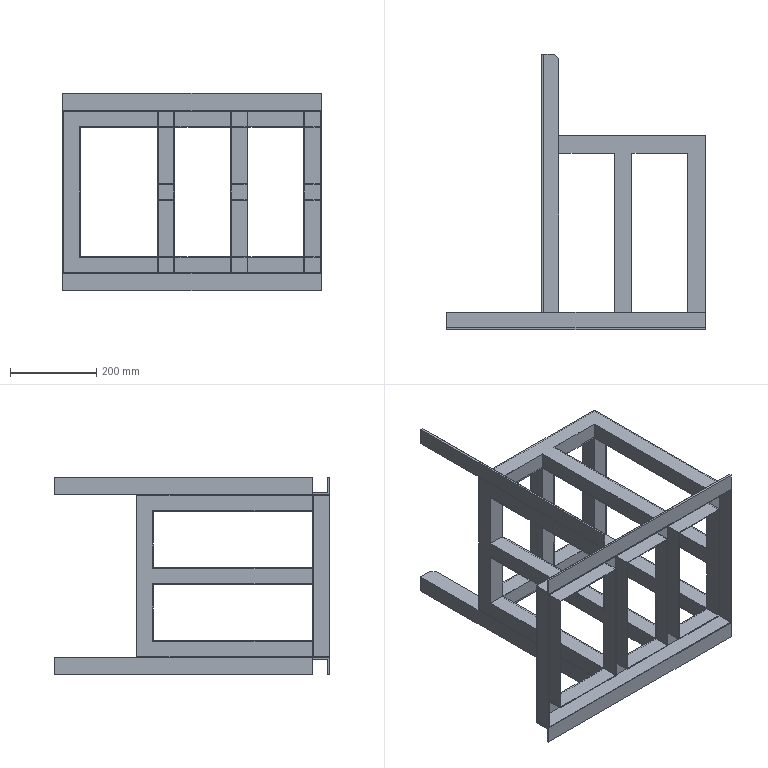Part | STEP file | Produce dryer line heating fan-SIROCCOFAN-3KW-101 | 5 solids | 162 faces | box 600 x 640 x 460 mm | volume 2910476 mm3 | plane 162